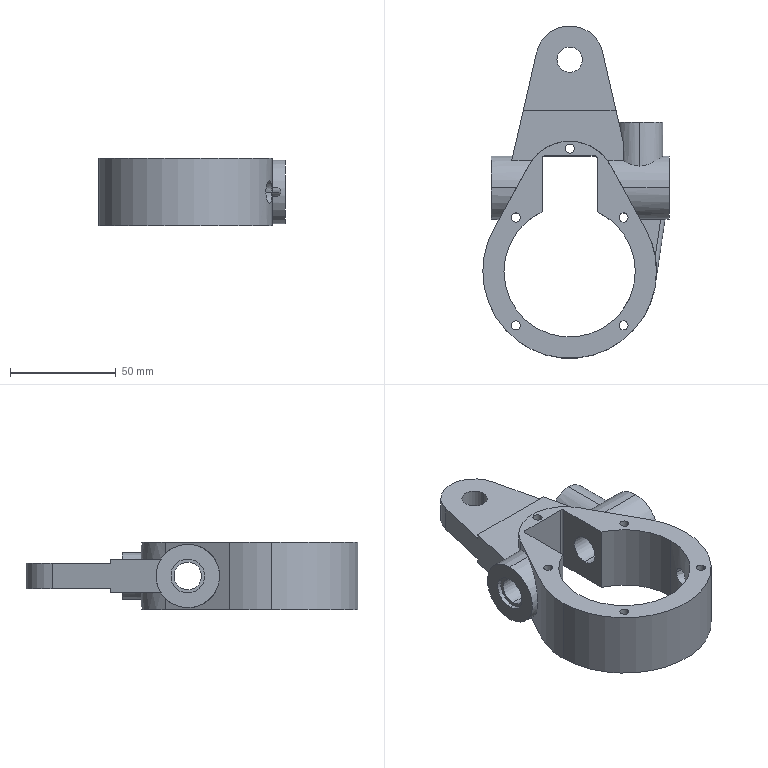Part | SolidWorks | features ICE 9, HoleWzd 4, CirPattern 1, Extrusion 1, Fillet 1, RefAxis 1, RevCut 1 | 1 solid | 67 faces | box 88 x 157 x 32 mm | volume 127446 mm3 | cylinder 41 | plane 24 | cone 2 | commonest cylinder face diameters 4.3 x10 30 x4 82 x4 22 x3 62 x3 2 x2